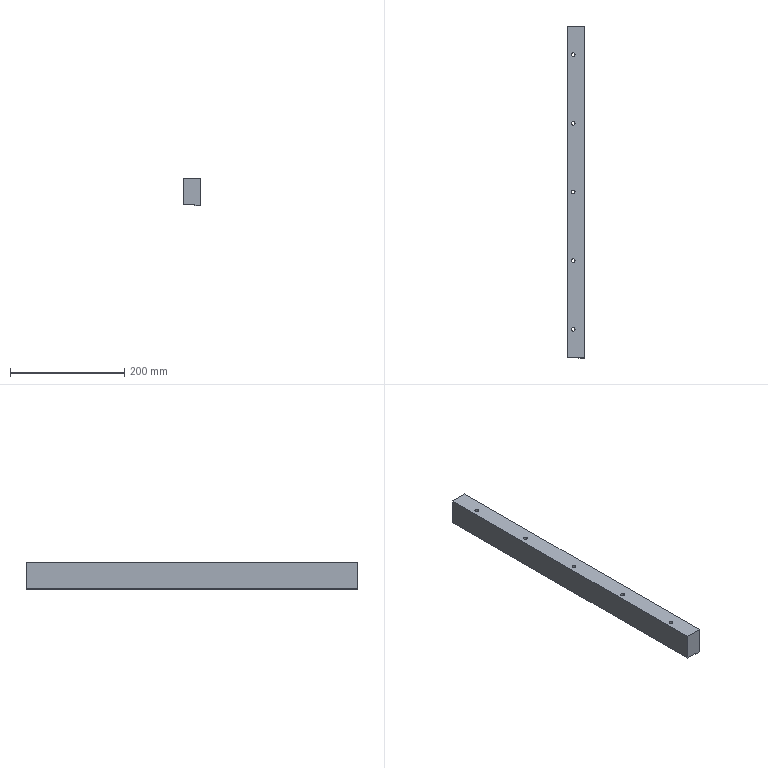Part | SolidWorks | features HoleWzd 2, LPattern 2, Extrusion 1, ICE 1 | 1 solid | 73 faces | box 30 x 580 x 48 mm | volume 800287 mm3 | cylinder 40 | cone 20 | plane 13 | commonest cylinder face diameters 4.2 x20 6.6 x10 11 x10